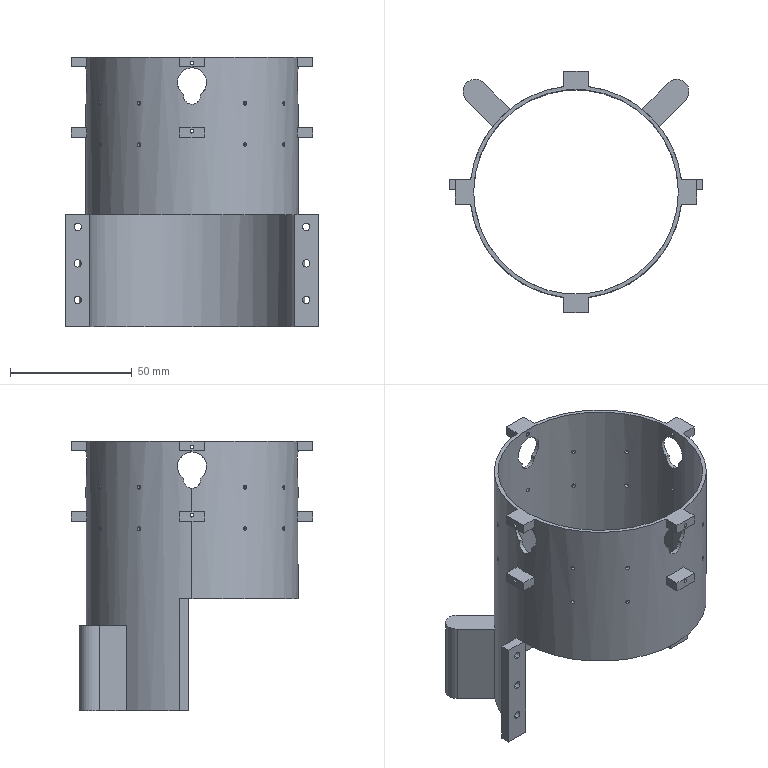Part | SolidWorks | features ICE 12, CirPattern 4, Fillet 2, HoleWzd 2, Extrusion 1 | 1 solid | 144 faces | box 104 x 99.2 x 110.99 mm | volume 51523 mm3 | cylinder 89 | plane 55 | commonest cylinder face diameters 1.6 x48 3 x12 7 x9 12 x9 5 x4 10 x3